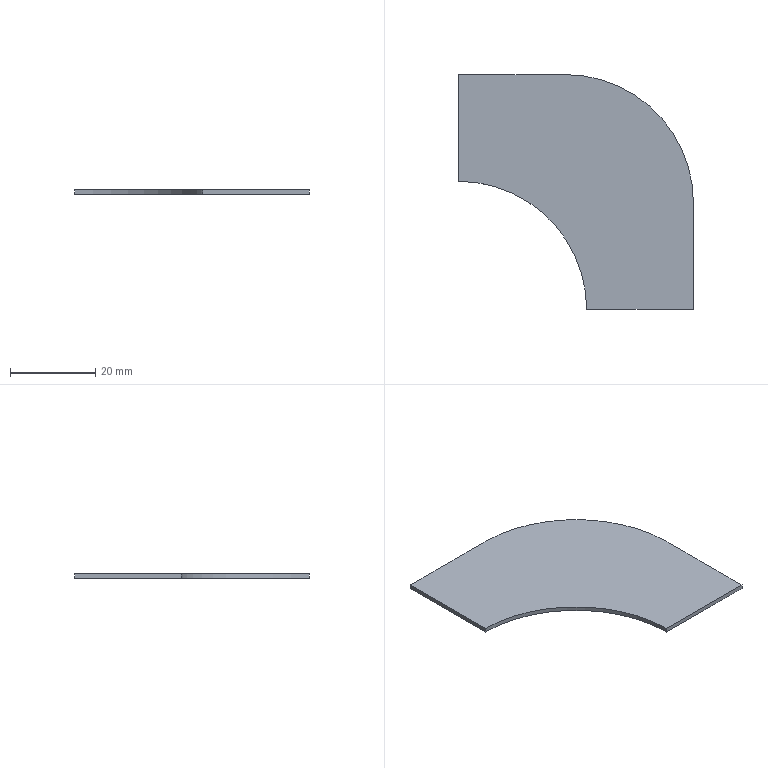Part | STEP file | HESS-408-70-15W-N-9-inner liner rounded corner | 1 solid | 8 faces | box 55 x 55 x 1 mm | volume 2125 mm3 | plane 6 | cylinder 2 | commonest cylinder face diameters 60 x2
STEP:
#1=CARTESIAN_POINT('',(0.,0.,0.));
#2=DIRECTION('',(0.,0.,1.));
#3=DIRECTION('',(1.,0.,0.));
#4=AXIS2_PLACEMENT_3D('',#1,#2,#3);
#5=CARTESIAN_POINT('',(30.,0.,-1.));
#6=VERTEX_POINT('',#5);
#7=CARTESIAN_POINT('',(0.,30.,-1.));
#8=VERTEX_POINT('',#7);
#9=CARTESIAN_POINT('',(0.,0.,-1.));
#10=DIRECTION('',(0.,0.,1.));
#11=DIRECTION('',(0.,-1.,0.));
#12=AXIS2_PLACEMENT_3D('',#9,#10,#11);
#13=CIRCLE('',#12,30.);
#14=CARTESIAN_POINT('',(25.,25.,-1.));
#15=DIRECTION('',(0.,0.,-1.));
#16=DIRECTION('',(0.,1.,0.));
#17=AXIS2_PLACEMENT_3D('',#14,#15,#16);
#18=PLANE('',#17);
#19=CARTESIAN_POINT('',(-55.,-25.));
#20=CARTESIAN_POINT('',(-55.,26.962));
#21=CARTESIAN_POINT('',(-10.,0.9808));
#22=CARTESIAN_POINT('',(35.,-25.));
#23=CARTESIAN_POINT('',(-10.,-50.981));
#24=CARTESIAN_POINT('',(-55.,-76.962));
#25=CARTESIAN_POINT('',(-55.,-25.));
#26=(BOUNDED_CURVE()B_SPLINE_CURVE(2,(#19,#20,#21,#22,#23,#24,#25),.UNSPECIFIED.,.T.,.F.)B_SPLINE_CURVE_WITH_KNOTS((1,2,2,2,2,1),(-2.094,0.,2.094,4.189,6.283,8.378),.UNSPECIFIED.)CURVE()GEOMETRIC_REPRESENTATION_ITEM()RATIONAL_B_SPLINE_CURVE((1.,0.5,1.,0.5,1.,0.5,1.))REPRESENTATION_ITEM(''));
#27=(GEOMETRIC_REPRESENTATION_CONTEXT(2)PARAMETRIC_REPRESENTATION_CONTEXT()REPRESENTATION_CONTEXT('',''));
#28=DEFINITIONAL_REPRESENTATION('',(#26),#27);
#29=PCURVE('',#18,#28);
#30=CARTESIAN_POINT('',(0.,0.,-1.));
#31=DIRECTION('',(0.,0.,1.));
#32=DIRECTION('',(0.,-1.,0.));
#33=AXIS2_PLACEMENT_3D('',#30,#31,#32);
#34=CYLINDRICAL_SURFACE('',#33,30.);
#35=CARTESIAN_POINT('',(0.,0.));
#36=DIRECTION('',(1.,0.));
#37=VECTOR('',#36,1.);
#38=LINE('',#35,#37);
#39=(GEOMETRIC_REPRESENTATION_CONTEXT(2)PARAMETRIC_REPRESENTATION_CONTEXT()REPRESENTATION_CONTEXT('',''));
#40=DEFINITIONAL_REPRESENTATION('',(#38),#39);
#41=PCURVE('',#34,#40);
#42=SURFACE_CURVE('',#13,(#29,#41),.PCURVE_S1.);
#43=EDGE_CURVE('',#6,#8,#42,.T.);
#44=ORIENTED_EDGE('',*,*,#43,.T.);
#45=CARTESIAN_POINT('',(0.,55.,-1.));
#46=VERTEX_POINT('',#45);
#47=CARTESIAN_POINT('',(0.,25.,-1.));
#48=DIRECTION('',(0.,1.,0.));
#49=VECTOR('',#48,1.);
#50=LINE('',#47,#49);
#51=CARTESIAN_POINT('',(0.,-25.));
#52=DIRECTION('',(1.,0.));
#53=VECTOR('',#52,1.);
#54=LINE('',#51,#53);
#55=(GEOMETRIC_REPRESENTATION_CONTEXT(2)PARAMETRIC_REPRESENTATION_CONTEXT()REPRESENTATION_CONTEXT('',''));
#56=DEFINITIONAL_REPRESENTATION('',(#54),#55);
#57=PCURVE('',#18,#56);
#58=CARTESIAN_POINT('',(0.,30.,-1.));
#59=DIRECTION('',(-1.,0.,0.));
#60=DIRECTION('',(0.,-1.,0.));
#61=AXIS2_PLACEMENT_3D('',#58,#59,#60);
#62=PLANE('',#61);
#63=CARTESIAN_POINT('',(5.,0.));
#64=DIRECTION('',(-1.,0.));
#65=VECTOR('',#64,1.);
#66=LINE('',#63,#65);
#67=(GEOMETRIC_REPRESENTATION_CONTEXT(2)PARAMETRIC_REPRESENTATION_CONTEXT()REPRESENTATION_CONTEXT('',''));
#68=DEFINITIONAL_REPRESENTATION('',(#66),#67);
#69=PCURVE('',#62,#68);
#70=SURFACE_CURVE('',#50,(#57,#69),.PCURVE_S1.);
#71=EDGE_CURVE('',#8,#46,#70,.T.);
#72=ORIENTED_EDGE('',*,*,#71,.T.);
#73=CARTESIAN_POINT('',(25.,55.,-1.));
#74=VERTEX_POINT('',#73);
#75=CARTESIAN_POINT('',(25.,55.,-1.));
#76=DIRECTION('',(1.,0.,0.));
#77=VECTOR('',#76,1.);
#78=LINE('',#75,#77);
#79=CARTESIAN_POINT('',(30.,0.));
#80=DIRECTION('',(0.,1.));
#81=VECTOR('',#80,1.);
#82=LINE('',#79,#81);
#83=(GEOMETRIC_REPRESENTATION_CONTEXT(2)PARAMETRIC_REPRESENTATION_CONTEXT()REPRESENTATION_CONTEXT('',''));
#84=DEFINITIONAL_REPRESENTATION('',(#82),#83);
#85=PCURVE('',#18,#84);
#86=CARTESIAN_POINT('',(0.,55.,-1.));
#87=DIRECTION('',(0.,1.,0.));
#88=DIRECTION('',(-1.,0.,0.));
#89=AXIS2_PLACEMENT_3D('',#86,#87,#88);
#90=PLANE('',#89);
#91=CARTESIAN_POINT('',(-25.,0.));
#92=DIRECTION('',(-1.,0.));
#93=VECTOR('',#92,1.);
#94=LINE('',#91,#93);
#95=(GEOMETRIC_REPRESENTATION_CONTEXT(2)PARAMETRIC_REPRESENTATION_CONTEXT()REPRESENTATION_CONTEXT('',''));
#96=DEFINITIONAL_REPRESENTATION('',(#94),#95);
#97=PCURVE('',#90,#96);
#98=SURFACE_CURVE('',#78,(#85,#97),.PCURVE_S1.);
#99=EDGE_CURVE('',#46,#74,#98,.T.);
#100=ORIENTED_EDGE('',*,*,#99,.T.);
#101=CARTESIAN_POINT('',(55.,25.,-1.));
#102=VERTEX_POINT('',#101);
#103=CARTESIAN_POINT('',(25.,25.,-1.));
#104=DIRECTION('',(0.,0.,-1.));
#105=DIRECTION('',(0.,-1.,0.));
#106=AXIS2_PLACEMENT_3D('',#103,#104,#105);
#107=CIRCLE('',#106,30.);
#108=CARTESIAN_POINT('',(0.,0.));
#109=DIRECTION('',(-1.,0.));
#110=AXIS2_PLACEMENT_2D('',#108,#109);
#111=CIRCLE('',#110,30.);
#112=(GEOMETRIC_REPRESENTATION_CONTEXT(2)PARAMETRIC_REPRESENTATION_CONTEXT()REPRESENTATION_CONTEXT('',''));
#113=DEFINITIONAL_REPRESENTATION('',(#111),#112);
#114=PCURVE('',#18,#113);
#115=CARTESIAN_POINT('',(25.,25.,-1.));
#116=DIRECTION('',(0.,0.,1.));
#117=DIRECTION('',(0.,-1.,0.));
#118=AXIS2_PLACEMENT_3D('',#115,#116,#117);
#119=CYLINDRICAL_SURFACE('',#118,30.);
#120=CARTESIAN_POINT('',(6.283,0.));
#121=DIRECTION('',(-1.,0.));
#122=VECTOR('',#121,1.);
#123=LINE('',#120,#122);
#124=(GEOMETRIC_REPRESENTATION_CONTEXT(2)PARAMETRIC_REPRESENTATION_CONTEXT()REPRESENTATION_CONTEXT('',''));
#125=DEFINITIONAL_REPRESENTATION('',(#123),#124);
#126=PCURVE('',#119,#125);
#127=SURFACE_CURVE('',#107,(#114,#126),.PCURVE_S1.);
#128=EDGE_CURVE('',#74,#102,#127,.T.);
#129=ORIENTED_EDGE('',*,*,#128,.T.);
#130=CARTESIAN_POINT('',(55.,0.,-1.));
#131=VERTEX_POINT('',#130);
#132=CARTESIAN_POINT('',(55.,25.,-1.));
#133=DIRECTION('',(0.,-1.,0.));
#134=VECTOR('',#133,1.);
#135=LINE('',#132,#134);
#136=CARTESIAN_POINT('',(0.,30.));
#137=DIRECTION('',(-1.,0.));
#138=VECTOR('',#137,1.);
#139=LINE('',#136,#138);
#140=(GEOMETRIC_REPRESENTATION_CONTEXT(2)PARAMETRIC_REPRESENTATION_CONTEXT()REPRESENTATION_CONTEXT('',''));
#141=DEFINITIONAL_REPRESENTATION('',(#139),#140);
#142=PCURVE('',#18,#141);
#143=CARTESIAN_POINT('',(55.,0.,-1.));
#144=DIRECTION('',(1.,0.,0.));
#145=DIRECTION('',(0.,1.,0.));
#146=AXIS2_PLACEMENT_3D('',#143,#144,#145);
#147=PLANE('',#146);
#148=CARTESIAN_POINT('',(25.,0.));
#149=DIRECTION('',(-1.,0.));
#150=VECTOR('',#149,1.);
#151=LINE('',#148,#150);
#152=(GEOMETRIC_REPRESENTATION_CONTEXT(2)PARAMETRIC_REPRESENTATION_CONTEXT()REPRESENTATION_CONTEXT('',''));
#153=DEFINITIONAL_REPRESENTATION('',(#151),#152);
#154=PCURVE('',#147,#153);
#155=SURFACE_CURVE('',#135,(#142,#154),.PCURVE_S1.);
#156=EDGE_CURVE('',#102,#131,#155,.T.);
#157=ORIENTED_EDGE('',*,*,#156,.T.);
#158=CARTESIAN_POINT('',(25.,0.,-1.));
#159=DIRECTION('',(-1.,0.,0.));
#160=VECTOR('',#159,1.);
#161=LINE('',#158,#160);
#162=CARTESIAN_POINT('',(-25.,0.));
#163=DIRECTION('',(0.,-1.));
#164=VECTOR('',#163,1.);
#165=LINE('',#162,#164);
#166=(GEOMETRIC_REPRESENTATION_CONTEXT(2)PARAMETRIC_REPRESENTATION_CONTEXT()REPRESENTATION_CONTEXT('',''));
#167=DEFINITIONAL_REPRESENTATION('',(#165),#166);
#168=PCURVE('',#18,#167);
#169=CARTESIAN_POINT('',(30.,0.,-1.));
#170=DIRECTION('',(0.,-1.,0.));
#171=DIRECTION('',(0.,0.,-1.));
#172=AXIS2_PLACEMENT_3D('',#169,#170,#171);
#173=PLANE('',#172);
#174=CARTESIAN_POINT('',(0.,-5.));
#175=DIRECTION('',(0.,-1.));
#176=VECTOR('',#175,1.);
#177=LINE('',#174,#176);
#178=(GEOMETRIC_REPRESENTATION_CONTEXT(2)PARAMETRIC_REPRESENTATION_CONTEXT()REPRESENTATION_CONTEXT('',''));
#179=DEFINITIONAL_REPRESENTATION('',(#177),#178);
#180=PCURVE('',#173,#179);
#181=SURFACE_CURVE('',#161,(#168,#180),.PCURVE_S1.);
#182=EDGE_CURVE('',#131,#6,#181,.T.);
#183=ORIENTED_EDGE('',*,*,#182,.T.);
#184=EDGE_LOOP('',(#44,#72,#100,#129,#157,#183));
#185=FACE_BOUND('',#184,.T.);
#186=ADVANCED_FACE('',(#185),#18,.T.);
#187=ORIENTED_EDGE('',*,*,#71,.F.);
#188=CARTESIAN_POINT('',(0.,30.,0.));
#189=VERTEX_POINT('',#188);
#190=CARTESIAN_POINT('',(0.,30.,-1.));
#191=DIRECTION('',(0.,0.,1.));
#192=VECTOR('',#191,1.);
#193=LINE('',#190,#192);
#194=CARTESIAN_POINT('',(0.,0.));
#195=DIRECTION('',(0.,1.));
#196=VECTOR('',#195,1.);
#197=LINE('',#194,#196);
#198=(GEOMETRIC_REPRESENTATION_CONTEXT(2)PARAMETRIC_REPRESENTATION_CONTEXT()REPRESENTATION_CONTEXT('',''));
#199=DEFINITIONAL_REPRESENTATION('',(#197),#198);
#200=PCURVE('',#62,#199);
#201=CARTESIAN_POINT('',(3.142,0.));
#202=DIRECTION('',(0.,1.));
#203=VECTOR('',#202,1.);
#204=LINE('',#201,#203);
#205=(GEOMETRIC_REPRESENTATION_CONTEXT(2)PARAMETRIC_REPRESENTATION_CONTEXT()REPRESENTATION_CONTEXT('',''));
#206=DEFINITIONAL_REPRESENTATION('',(#204),#205);
#207=PCURVE('',#34,#206);
#208=SURFACE_CURVE('',#193,(#200,#207),.PCURVE_S1.);
#209=EDGE_CURVE('',#8,#189,#208,.T.);
#210=ORIENTED_EDGE('',*,*,#209,.T.);
#211=CARTESIAN_POINT('',(0.,55.,0.));
#212=VERTEX_POINT('',#211);
#213=CARTESIAN_POINT('',(0.,30.,0.));
#214=DIRECTION('',(0.,1.,0.));
#215=VECTOR('',#214,1.);
#216=LINE('',#213,#215);
#217=CARTESIAN_POINT('',(0.,1.));
#218=DIRECTION('',(-1.,0.));
#219=VECTOR('',#218,1.);
#220=LINE('',#217,#219);
#221=(GEOMETRIC_REPRESENTATION_CONTEXT(2)PARAMETRIC_REPRESENTATION_CONTEXT()REPRESENTATION_CONTEXT('',''));
#222=DEFINITIONAL_REPRESENTATION('',(#220),#221);
#223=PCURVE('',#62,#222);
#224=CARTESIAN_POINT('',(25.,25.,0.));
#225=DIRECTION('',(0.,0.,-1.));
#226=DIRECTION('',(0.,1.,0.));
#227=AXIS2_PLACEMENT_3D('',#224,#225,#226);
#228=PLANE('',#227);
#229=CARTESIAN_POINT('',(5.,-25.));
#230=DIRECTION('',(1.,0.));
#231=VECTOR('',#230,1.);
#232=LINE('',#229,#231);
#233=(GEOMETRIC_REPRESENTATION_CONTEXT(2)PARAMETRIC_REPRESENTATION_CONTEXT()REPRESENTATION_CONTEXT('',''));
#234=DEFINITIONAL_REPRESENTATION('',(#232),#233);
#235=PCURVE('',#228,#234);
#236=SURFACE_CURVE('',#216,(#223,#235),.PCURVE_S1.);
#237=EDGE_CURVE('',#189,#212,#236,.T.);
#238=ORIENTED_EDGE('',*,*,#237,.T.);
#239=CARTESIAN_POINT('',(0.,55.,-1.));
#240=DIRECTION('',(0.,0.,-1.));
#241=VECTOR('',#240,1.);
#242=LINE('',#239,#241);
#243=CARTESIAN_POINT('',(-25.,0.));
#244=DIRECTION('',(0.,-1.));
#245=VECTOR('',#244,1.);
#246=LINE('',#243,#245);
#247=(GEOMETRIC_REPRESENTATION_CONTEXT(2)PARAMETRIC_REPRESENTATION_CONTEXT()REPRESENTATION_CONTEXT('',''));
#248=DEFINITIONAL_REPRESENTATION('',(#246),#247);
#249=PCURVE('',#62,#248);
#250=CARTESIAN_POINT('',(0.,0.));
#251=DIRECTION('',(0.,-1.));
#252=VECTOR('',#251,1.);
#253=LINE('',#250,#252);
#254=(GEOMETRIC_REPRESENTATION_CONTEXT(2)PARAMETRIC_REPRESENTATION_CONTEXT()REPRESENTATION_CONTEXT('',''));
#255=DEFINITIONAL_REPRESENTATION('',(#253),#254);
#256=PCURVE('',#90,#255);
#257=SURFACE_CURVE('',#242,(#249,#256),.PCURVE_S1.);
#258=EDGE_CURVE('',#212,#46,#257,.T.);
#259=ORIENTED_EDGE('',*,*,#258,.T.);
#260=EDGE_LOOP('',(#187,#210,#238,#259));
#261=FACE_BOUND('',#260,.T.);
#262=ADVANCED_FACE('',(#261),#62,.T.);
#263=CARTESIAN_POINT('',(30.,0.,0.));
#264=VERTEX_POINT('',#263);
#265=CARTESIAN_POINT('',(0.,0.,0.));
#266=DIRECTION('',(0.,0.,-1.));
#267=DIRECTION('',(0.,-1.,0.));
#268=AXIS2_PLACEMENT_3D('',#265,#266,#267);
#269=CIRCLE('',#268,30.);
#270=CARTESIAN_POINT('',(6.283,1.));
#271=DIRECTION('',(-1.,0.));
#272=VECTOR('',#271,1.);
#273=LINE('',#270,#272);
#274=(GEOMETRIC_REPRESENTATION_CONTEXT(2)PARAMETRIC_REPRESENTATION_CONTEXT()REPRESENTATION_CONTEXT('',''));
#275=DEFINITIONAL_REPRESENTATION('',(#273),#274);
#276=PCURVE('',#34,#275);
#277=CARTESIAN_POINT('',(-25.,-25.));
#278=DIRECTION('',(-1.,0.));
#279=AXIS2_PLACEMENT_2D('',#277,#278);
#280=CIRCLE('',#279,30.);
#281=(GEOMETRIC_REPRESENTATION_CONTEXT(2)PARAMETRIC_REPRESENTATION_CONTEXT()REPRESENTATION_CONTEXT('',''));
#282=DEFINITIONAL_REPRESENTATION('',(#280),#281);
#283=PCURVE('',#228,#282);
#284=SURFACE_CURVE('',#269,(#276,#283),.PCURVE_S1.);
#285=EDGE_CURVE('',#189,#264,#284,.T.);
#286=ORIENTED_EDGE('',*,*,#285,.T.);
#287=CARTESIAN_POINT('',(30.,0.,-1.));
#288=DIRECTION('',(0.,0.,-1.));
#289=VECTOR('',#288,1.);
#290=LINE('',#287,#289);
#291=CARTESIAN_POINT('',(1.571,0.));
#292=DIRECTION('',(0.,-1.));
#293=VECTOR('',#292,1.);
#294=LINE('',#291,#293);
#295=(GEOMETRIC_REPRESENTATION_CONTEXT(2)PARAMETRIC_REPRESENTATION_CONTEXT()REPRESENTATION_CONTEXT('',''));
#296=DEFINITIONAL_REPRESENTATION('',(#294),#295);
#297=PCURVE('',#34,#296);
#298=CARTESIAN_POINT('',(0.,0.));
#299=DIRECTION('',(1.,0.));
#300=VECTOR('',#299,1.);
#301=LINE('',#298,#300);
#302=(GEOMETRIC_REPRESENTATION_CONTEXT(2)PARAMETRIC_REPRESENTATION_CONTEXT()REPRESENTATION_CONTEXT('',''));
#303=DEFINITIONAL_REPRESENTATION('',(#301),#302);
#304=PCURVE('',#173,#303);
#305=SURFACE_CURVE('',#290,(#297,#304),.PCURVE_S1.);
#306=EDGE_CURVE('',#264,#6,#305,.T.);
#307=ORIENTED_EDGE('',*,*,#306,.T.);
#308=ORIENTED_EDGE('',*,*,#43,.T.);
#309=ORIENTED_EDGE('',*,*,#209,.T.);
#310=EDGE_LOOP('',(#286,#307,#308,#309));
#311=FACE_BOUND('',#310,.F.);
#312=ADVANCED_FACE('',(#311),#34,.F.);
#313=ORIENTED_EDGE('',*,*,#182,.F.);
#314=CARTESIAN_POINT('',(55.,0.,0.));
#315=VERTEX_POINT('',#314);
#316=CARTESIAN_POINT('',(55.,0.,-1.));
#317=DIRECTION('',(0.,0.,1.));
#318=VECTOR('',#317,1.);
#319=LINE('',#316,#318);
#320=CARTESIAN_POINT('',(0.,25.));
#321=DIRECTION('',(-1.,0.));
#322=VECTOR('',#321,1.);
#323=LINE('',#320,#322);
#324=(GEOMETRIC_REPRESENTATION_CONTEXT(2)PARAMETRIC_REPRESENTATION_CONTEXT()REPRESENTATION_CONTEXT('',''));
#325=DEFINITIONAL_REPRESENTATION('',(#323),#324);
#326=PCURVE('',#173,#325);
#327=CARTESIAN_POINT('',(0.,0.));
#328=DIRECTION('',(0.,1.));
#329=VECTOR('',#328,1.);
#330=LINE('',#327,#329);
#331=(GEOMETRIC_REPRESENTATION_CONTEXT(2)PARAMETRIC_REPRESENTATION_CONTEXT()REPRESENTATION_CONTEXT('',''));
#332=DEFINITIONAL_REPRESENTATION('',(#330),#331);
#333=PCURVE('',#147,#332);
#334=SURFACE_CURVE('',#319,(#326,#333),.PCURVE_S1.);
#335=EDGE_CURVE('',#131,#315,#334,.T.);
#336=ORIENTED_EDGE('',*,*,#335,.T.);
#337=CARTESIAN_POINT('',(30.,0.,0.));
#338=DIRECTION('',(-1.,0.,0.));
#339=VECTOR('',#338,1.);
#340=LINE('',#337,#339);
#341=CARTESIAN_POINT('',(-1.,0.));
#342=DIRECTION('',(0.,-1.));
#343=VECTOR('',#342,1.);
#344=LINE('',#341,#343);
#345=(GEOMETRIC_REPRESENTATION_CONTEXT(2)PARAMETRIC_REPRESENTATION_CONTEXT()REPRESENTATION_CONTEXT('',''));
#346=DEFINITIONAL_REPRESENTATION('',(#344),#345);
#347=PCURVE('',#173,#346);
#348=CARTESIAN_POINT('',(-25.,5.));
#349=DIRECTION('',(0.,-1.));
#350=VECTOR('',#349,1.);
#351=LINE('',#348,#350);
#352=(GEOMETRIC_REPRESENTATION_CONTEXT(2)PARAMETRIC_REPRESENTATION_CONTEXT()REPRESENTATION_CONTEXT('',''));
#353=DEFINITIONAL_REPRESENTATION('',(#351),#352);
#354=PCURVE('',#228,#353);
#355=SURFACE_CURVE('',#340,(#347,#354),.PCURVE_S1.);
#356=EDGE_CURVE('',#315,#264,#355,.T.);
#357=ORIENTED_EDGE('',*,*,#356,.T.);
#358=ORIENTED_EDGE('',*,*,#306,.T.);
#359=EDGE_LOOP('',(#313,#336,#357,#358));
#360=FACE_BOUND('',#359,.T.);
#361=ADVANCED_FACE('',(#360),#173,.T.);
#362=ORIENTED_EDGE('',*,*,#156,.F.);
#363=CARTESIAN_POINT('',(55.,25.,0.));
#364=VERTEX_POINT('',#363);
#365=CARTESIAN_POINT('',(55.,25.,-1.));
#366=DIRECTION('',(0.,0.,1.));
#367=VECTOR('',#366,1.);
#368=LINE('',#365,#367);
#369=CARTESIAN_POINT('',(25.,0.));
#370=DIRECTION('',(0.,1.));
#371=VECTOR('',#370,1.);
#372=LINE('',#369,#371);
#373=(GEOMETRIC_REPRESENTATION_CONTEXT(2)PARAMETRIC_REPRESENTATION_CONTEXT()REPRESENTATION_CONTEXT('',''));
#374=DEFINITIONAL_REPRESENTATION('',(#372),#373);
#375=PCURVE('',#147,#374);
#376=CARTESIAN_POINT('',(1.571,0.));
#377=DIRECTION('',(0.,1.));
#378=VECTOR('',#377,1.);
#379=LINE('',#376,#378);
#380=(GEOMETRIC_REPRESENTATION_CONTEXT(2)PARAMETRIC_REPRESENTATION_CONTEXT()REPRESENTATION_CONTEXT('',''));
#381=DEFINITIONAL_REPRESENTATION('',(#379),#380);
#382=PCURVE('',#119,#381);
#383=SURFACE_CURVE('',#368,(#375,#382),.PCURVE_S1.);
#384=EDGE_CURVE('',#102,#364,#383,.T.);
#385=ORIENTED_EDGE('',*,*,#384,.T.);
#386=CARTESIAN_POINT('',(55.,0.,0.));
#387=DIRECTION('',(0.,-1.,0.));
#388=VECTOR('',#387,1.);
#389=LINE('',#386,#388);
#390=CARTESIAN_POINT('',(0.,1.));
#391=DIRECTION('',(-1.,0.));
#392=VECTOR('',#391,1.);
#393=LINE('',#390,#392);
#394=(GEOMETRIC_REPRESENTATION_CONTEXT(2)PARAMETRIC_REPRESENTATION_CONTEXT()REPRESENTATION_CONTEXT('',''));
#395=DEFINITIONAL_REPRESENTATION('',(#393),#394);
#396=PCURVE('',#147,#395);
#397=CARTESIAN_POINT('',(-25.,30.));
#398=DIRECTION('',(-1.,0.));
#399=VECTOR('',#398,1.);
#400=LINE('',#397,#399);
#401=(GEOMETRIC_REPRESENTATION_CONTEXT(2)PARAMETRIC_REPRESENTATION_CONTEXT()REPRESENTATION_CONTEXT('',''));
#402=DEFINITIONAL_REPRESENTATION('',(#400),#401);
#403=PCURVE('',#228,#402);
#404=SURFACE_CURVE('',#389,(#396,#403),.PCURVE_S1.);
#405=EDGE_CURVE('',#364,#315,#404,.T.);
#406=ORIENTED_EDGE('',*,*,#405,.T.);
#407=ORIENTED_EDGE('',*,*,#335,.F.);
#408=EDGE_LOOP('',(#362,#385,#406,#407));
#409=FACE_BOUND('',#408,.T.);
#410=ADVANCED_FACE('',(#409),#147,.T.);
#411=ORIENTED_EDGE('',*,*,#128,.F.);
#412=CARTESIAN_POINT('',(25.,55.,0.));
#413=VERTEX_POINT('',#412);
#414=CARTESIAN_POINT('',(25.,55.,-1.));
#415=DIRECTION('',(0.,0.,1.));
#416=VECTOR('',#415,1.);
#417=LINE('',#414,#416);
#418=CARTESIAN_POINT('',(3.142,0.));
#419=DIRECTION('',(0.,1.));
#420=VECTOR('',#419,1.);
#421=LINE('',#418,#420);
#422=(GEOMETRIC_REPRESENTATION_CONTEXT(2)PARAMETRIC_REPRESENTATION_CONTEXT()REPRESENTATION_CONTEXT('',''));
#423=DEFINITIONAL_REPRESENTATION('',(#421),#422);
#424=PCURVE('',#119,#423);
#425=CARTESIAN_POINT('',(-25.,0.));
#426=DIRECTION('',(0.,1.));
#427=VECTOR('',#426,1.);
#428=LINE('',#425,#427);
#429=(GEOMETRIC_REPRESENTATION_CONTEXT(2)PARAMETRIC_REPRESENTATION_CONTEXT()REPRESENTATION_CONTEXT('',''));
#430=DEFINITIONAL_REPRESENTATION('',(#428),#429);
#431=PCURVE('',#90,#430);
#432=SURFACE_CURVE('',#417,(#424,#431),.PCURVE_S1.);
#433=EDGE_CURVE('',#74,#413,#432,.T.);
#434=ORIENTED_EDGE('',*,*,#433,.T.);
#435=CARTESIAN_POINT('',(25.,25.,0.));
#436=DIRECTION('',(0.,0.,-1.));
#437=DIRECTION('',(0.,-1.,0.));
#438=AXIS2_PLACEMENT_3D('',#435,#436,#437);
#439=CIRCLE('',#438,30.);
#440=CARTESIAN_POINT('',(6.283,1.));
#441=DIRECTION('',(-1.,0.));
#442=VECTOR('',#441,1.);
#443=LINE('',#440,#442);
#444=(GEOMETRIC_REPRESENTATION_CONTEXT(2)PARAMETRIC_REPRESENTATION_CONTEXT()REPRESENTATION_CONTEXT('',''));
#445=DEFINITIONAL_REPRESENTATION('',(#443),#444);
#446=PCURVE('',#119,#445);
#447=CARTESIAN_POINT('',(0.,0.));
#448=DIRECTION('',(-1.,0.));
#449=AXIS2_PLACEMENT_2D('',#447,#448);
#450=CIRCLE('',#449,30.);
#451=(GEOMETRIC_REPRESENTATION_CONTEXT(2)PARAMETRIC_REPRESENTATION_CONTEXT()REPRESENTATION_CONTEXT('',''));
#452=DEFINITIONAL_REPRESENTATION('',(#450),#451);
#453=PCURVE('',#228,#452);
#454=SURFACE_CURVE('',#439,(#446,#453),.PCURVE_S1.);
#455=EDGE_CURVE('',#413,#364,#454,.T.);
#456=ORIENTED_EDGE('',*,*,#455,.T.);
#457=ORIENTED_EDGE('',*,*,#384,.F.);
#458=EDGE_LOOP('',(#411,#434,#456,#457));
#459=FACE_BOUND('',#458,.T.);
#460=ADVANCED_FACE('',(#459),#119,.T.);
#461=ORIENTED_EDGE('',*,*,#99,.F.);
#462=ORIENTED_EDGE('',*,*,#258,.F.);
#463=CARTESIAN_POINT('',(0.,55.,0.));
#464=DIRECTION('',(1.,0.,0.));
#465=VECTOR('',#464,1.);
#466=LINE('',#463,#465);
#467=CARTESIAN_POINT('',(0.,1.));
#468=DIRECTION('',(-1.,0.));
#469=VECTOR('',#468,1.);
#470=LINE('',#467,#469);
#471=(GEOMETRIC_REPRESENTATION_CONTEXT(2)PARAMETRIC_REPRESENTATION_CONTEXT()REPRESENTATION_CONTEXT('',''));
#472=DEFINITIONAL_REPRESENTATION('',(#470),#471);
#473=PCURVE('',#90,#472);
#474=CARTESIAN_POINT('',(30.,-25.));
#475=DIRECTION('',(0.,1.));
#476=VECTOR('',#475,1.);
#477=LINE('',#474,#476);
#478=(GEOMETRIC_REPRESENTATION_CONTEXT(2)PARAMETRIC_REPRESENTATION_CONTEXT()REPRESENTATION_CONTEXT('',''));
#479=DEFINITIONAL_REPRESENTATION('',(#477),#478);
#480=PCURVE('',#228,#479);
#481=SURFACE_CURVE('',#466,(#473,#480),.PCURVE_S1.);
#482=EDGE_CURVE('',#212,#413,#481,.T.);
#483=ORIENTED_EDGE('',*,*,#482,.T.);
#484=ORIENTED_EDGE('',*,*,#433,.F.);
#485=EDGE_LOOP('',(#461,#462,#483,#484));
#486=FACE_BOUND('',#485,.T.);
#487=ADVANCED_FACE('',(#486),#90,.T.);
#488=ORIENTED_EDGE('',*,*,#237,.F.);
#489=ORIENTED_EDGE('',*,*,#285,.T.);
#490=ORIENTED_EDGE('',*,*,#356,.F.);
#491=ORIENTED_EDGE('',*,*,#405,.F.);
#492=ORIENTED_EDGE('',*,*,#455,.F.);
#493=ORIENTED_EDGE('',*,*,#482,.F.);
#494=EDGE_LOOP('',(#488,#489,#490,#491,#492,#493));
#495=FACE_BOUND('',#494,.T.);
#496=ADVANCED_FACE('',(#495),#228,.F.);
#497=CLOSED_SHELL('',(#186,#262,#312,#361,#410,#460,#487,#496));
#498=MANIFOLD_SOLID_BREP('',#497);
#499=(LENGTH_UNIT()NAMED_UNIT(*)SI_UNIT(.MILLI.,.METRE.));
#500=UNCERTAINTY_MEASURE_WITH_UNIT(LENGTH_MEASURE(0.0000001),#499,'','');
#501=(NAMED_UNIT(*)PLANE_ANGLE_UNIT()SI_UNIT($,.RADIAN.));
#502=(NAMED_UNIT(*)SI_UNIT($,.STERADIAN.)SOLID_ANGLE_UNIT());
#503=(GEOMETRIC_REPRESENTATION_CONTEXT(3)GLOBAL_UNCERTAINTY_ASSIGNED_CONTEXT((#500))GLOBAL_UNIT_ASSIGNED_CONTEXT((#499,#501,#502))REPRESENTATION_CONTEXT('',''));
#504=ADVANCED_BREP_SHAPE_REPRESENTATION('',(#4,#498),#503);